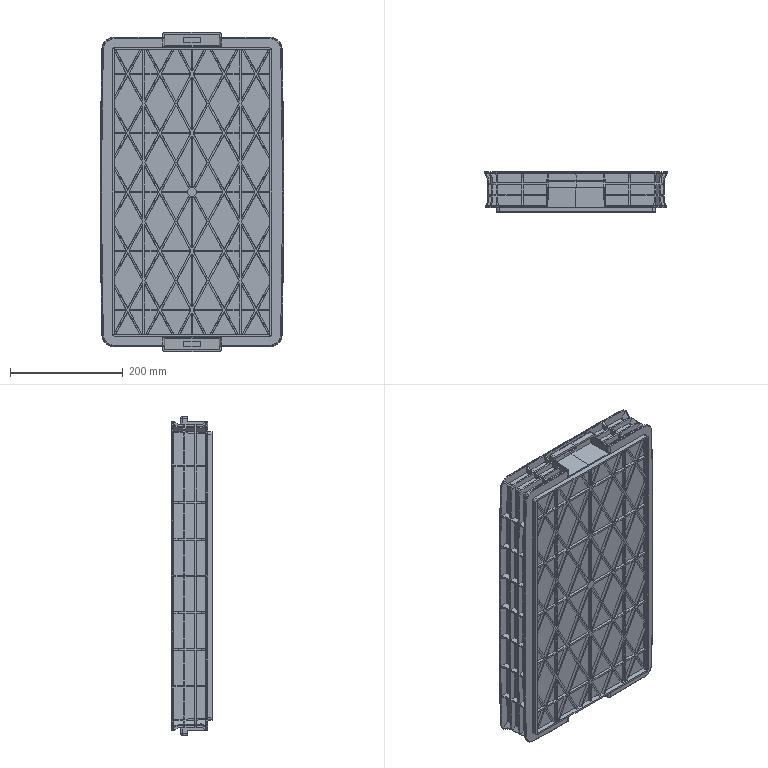Part | SolidWorks | 3 solids | 2068 faces | box 324.683 x 71 x 565.23 mm | volume 1531688 mm3 | plane 1303 | cylinder 417 | spline 206 | cone 89 | torus 49 | sphere 4 | commonest cylinder face diameters 4 x100 2 x72 1 x66 0.3 x48 79 x48 50 x24